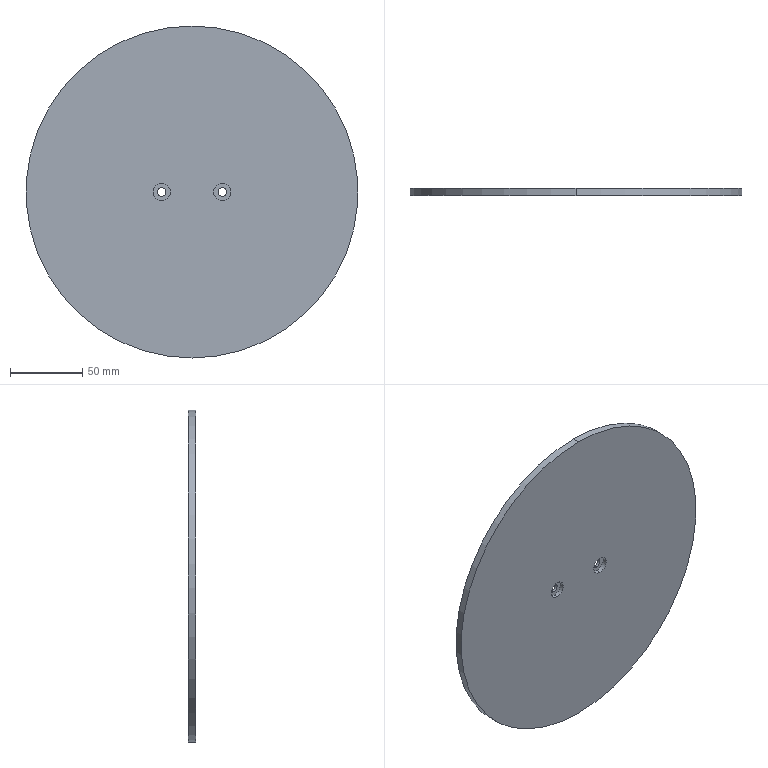Part | STEP file | Bottom cover | 1 solid | 14 faces | box 230 x 5 x 230 mm | volume 206946 mm3 | cylinder 10 | plane 4 | commonest cylinder face diameters 6 x4 12 x4 230 x2
STEP:
#1=CARTESIAN_POINT('',(21.,3.,6.));
#2=VERTEX_POINT('',#1);
#3=CARTESIAN_POINT('',(21.,3.,-6.));
#4=VERTEX_POINT('',#3);
#5=CARTESIAN_POINT('',(21.,3.,0.));
#6=DIRECTION('',(0.,-1.,0.));
#7=DIRECTION('',(0.,0.,-1.));
#8=AXIS2_PLACEMENT_3D('',#5,#6,#7);
#9=CIRCLE('',#8,6.);
#10=EDGE_CURVE('',#2,#4,#9,.T.);
#11=ORIENTED_EDGE('',*,*,#10,.F.);
#12=CARTESIAN_POINT('',(21.,0.,6.));
#13=VERTEX_POINT('',#12);
#14=CARTESIAN_POINT('',(21.,3.,6.));
#15=DIRECTION('',(0.,-1.,0.));
#16=VECTOR('',#15,1000.);
#17=LINE('',#14,#16);
#18=EDGE_CURVE('',#2,#13,#17,.T.);
#19=ORIENTED_EDGE('',*,*,#18,.T.);
#20=CARTESIAN_POINT('',(21.,0.,-6.));
#21=VERTEX_POINT('',#20);
#22=CARTESIAN_POINT('',(21.,0.,0.));
#23=DIRECTION('',(0.,-1.,0.));
#24=DIRECTION('',(0.,0.,-1.));
#25=AXIS2_PLACEMENT_3D('',#22,#23,#24);
#26=CIRCLE('',#25,6.);
#27=EDGE_CURVE('',#13,#21,#26,.T.);
#28=ORIENTED_EDGE('',*,*,#27,.T.);
#29=CARTESIAN_POINT('',(21.,3.,-6.));
#30=DIRECTION('',(0.,-1.,0.));
#31=VECTOR('',#30,1000.);
#32=LINE('',#29,#31);
#33=EDGE_CURVE('',#4,#21,#32,.T.);
#34=ORIENTED_EDGE('',*,*,#33,.F.);
#35=EDGE_LOOP('',(#11,#19,#28,#34));
#36=FACE_OUTER_BOUND('',#35,.T.);
#37=CARTESIAN_POINT('',(21.,3.,0.));
#38=DIRECTION('',(0.,-1.,0.));
#39=DIRECTION('',(0.,0.,-1.));
#40=AXIS2_PLACEMENT_3D('',#37,#38,#39);
#41=CYLINDRICAL_SURFACE('',#40,6.);
#42=ADVANCED_FACE('',(#36),#41,.F.);
#43=CARTESIAN_POINT('',(-21.,3.,6.));
#44=VERTEX_POINT('',#43);
#45=CARTESIAN_POINT('',(-21.,3.,-6.));
#46=VERTEX_POINT('',#45);
#47=CARTESIAN_POINT('',(-21.,3.,0.));
#48=DIRECTION('',(0.,-1.,0.));
#49=DIRECTION('',(0.,0.,-1.));
#50=AXIS2_PLACEMENT_3D('',#47,#48,#49);
#51=CIRCLE('',#50,6.);
#52=EDGE_CURVE('',#44,#46,#51,.T.);
#53=ORIENTED_EDGE('',*,*,#52,.F.);
#54=CARTESIAN_POINT('',(-21.,0.,6.));
#55=VERTEX_POINT('',#54);
#56=CARTESIAN_POINT('',(-21.,3.,6.));
#57=DIRECTION('',(0.,-1.,0.));
#58=VECTOR('',#57,1000.);
#59=LINE('',#56,#58);
#60=EDGE_CURVE('',#44,#55,#59,.T.);
#61=ORIENTED_EDGE('',*,*,#60,.T.);
#62=CARTESIAN_POINT('',(-21.,0.,-6.));
#63=VERTEX_POINT('',#62);
#64=CARTESIAN_POINT('',(-21.,0.,0.));
#65=DIRECTION('',(0.,-1.,0.));
#66=DIRECTION('',(0.,0.,-1.));
#67=AXIS2_PLACEMENT_3D('',#64,#65,#66);
#68=CIRCLE('',#67,6.);
#69=EDGE_CURVE('',#55,#63,#68,.T.);
#70=ORIENTED_EDGE('',*,*,#69,.T.);
#71=CARTESIAN_POINT('',(-21.,3.,-6.));
#72=DIRECTION('',(0.,-1.,0.));
#73=VECTOR('',#72,1000.);
#74=LINE('',#71,#73);
#75=EDGE_CURVE('',#46,#63,#74,.T.);
#76=ORIENTED_EDGE('',*,*,#75,.F.);
#77=EDGE_LOOP('',(#53,#61,#70,#76));
#78=FACE_OUTER_BOUND('',#77,.T.);
#79=CARTESIAN_POINT('',(-21.,3.,0.));
#80=DIRECTION('',(0.,-1.,0.));
#81=DIRECTION('',(0.,0.,-1.));
#82=AXIS2_PLACEMENT_3D('',#79,#80,#81);
#83=CYLINDRICAL_SURFACE('',#82,6.);
#84=ADVANCED_FACE('',(#78),#83,.F.);
#85=CARTESIAN_POINT('',(0.,5.,115.));
#86=VERTEX_POINT('',#85);
#87=CARTESIAN_POINT('',(0.,5.,-115.));
#88=VERTEX_POINT('',#87);
#89=CARTESIAN_POINT('',(0.,5.,0.));
#90=DIRECTION('',(0.,1.,0.));
#91=DIRECTION('',(0.,0.,1.));
#92=AXIS2_PLACEMENT_3D('',#89,#90,#91);
#93=CIRCLE('',#92,115.);
#94=EDGE_CURVE('',#86,#88,#93,.T.);
#95=ORIENTED_EDGE('',*,*,#94,.F.);
#96=CARTESIAN_POINT('',(0.,0.,115.));
#97=VERTEX_POINT('',#96);
#98=CARTESIAN_POINT('',(0.,5.,115.));
#99=DIRECTION('',(0.,-1.,0.));
#100=VECTOR('',#99,1000.);
#101=LINE('',#98,#100);
#102=EDGE_CURVE('',#86,#97,#101,.T.);
#103=ORIENTED_EDGE('',*,*,#102,.T.);
#104=CARTESIAN_POINT('',(0.,0.,-115.));
#105=VERTEX_POINT('',#104);
#106=CARTESIAN_POINT('',(0.,0.,0.));
#107=DIRECTION('',(0.,1.,0.));
#108=DIRECTION('',(0.,0.,1.));
#109=AXIS2_PLACEMENT_3D('',#106,#107,#108);
#110=CIRCLE('',#109,115.);
#111=EDGE_CURVE('',#97,#105,#110,.T.);
#112=ORIENTED_EDGE('',*,*,#111,.T.);
#113=CARTESIAN_POINT('',(0.,5.,-115.));
#114=DIRECTION('',(0.,-1.,0.));
#115=VECTOR('',#114,1000.);
#116=LINE('',#113,#115);
#117=EDGE_CURVE('',#88,#105,#116,.T.);
#118=ORIENTED_EDGE('',*,*,#117,.F.);
#119=EDGE_LOOP('',(#95,#103,#112,#118));
#120=FACE_OUTER_BOUND('',#119,.T.);
#121=CARTESIAN_POINT('',(0.,5.,0.));
#122=DIRECTION('',(0.,-1.,0.));
#123=DIRECTION('',(0.,0.,-1.));
#124=AXIS2_PLACEMENT_3D('',#121,#122,#123);
#125=CYLINDRICAL_SURFACE('',#124,115.);
#126=ADVANCED_FACE('',(#120),#125,.T.);
#127=CARTESIAN_POINT('',(-21.,3.,-3.));
#128=VERTEX_POINT('',#127);
#129=CARTESIAN_POINT('',(-21.,3.,3.));
#130=VERTEX_POINT('',#129);
#131=CARTESIAN_POINT('',(-21.,3.,0.));
#132=DIRECTION('',(0.,1.,0.));
#133=DIRECTION('',(0.,0.,-1.));
#134=AXIS2_PLACEMENT_3D('',#131,#132,#133);
#135=CIRCLE('',#134,3.);
#136=EDGE_CURVE('',#128,#130,#135,.T.);
#137=ORIENTED_EDGE('',*,*,#136,.F.);
#138=CARTESIAN_POINT('',(-21.,5.,-3.));
#139=VERTEX_POINT('',#138);
#140=CARTESIAN_POINT('',(-21.,-15.,-3.));
#141=DIRECTION('',(0.,1.,0.));
#142=VECTOR('',#141,1000.);
#143=LINE('',#140,#142);
#144=EDGE_CURVE('',#128,#139,#143,.T.);
#145=ORIENTED_EDGE('',*,*,#144,.T.);
#146=CARTESIAN_POINT('',(-21.,5.,3.));
#147=VERTEX_POINT('',#146);
#148=CARTESIAN_POINT('',(-21.,5.,0.));
#149=DIRECTION('',(0.,1.,0.));
#150=DIRECTION('',(0.,0.,1.));
#151=AXIS2_PLACEMENT_3D('',#148,#149,#150);
#152=CIRCLE('',#151,3.);
#153=EDGE_CURVE('',#139,#147,#152,.T.);
#154=ORIENTED_EDGE('',*,*,#153,.T.);
#155=CARTESIAN_POINT('',(-21.,-15.,3.));
#156=DIRECTION('',(0.,1.,0.));
#157=VECTOR('',#156,1000.);
#158=LINE('',#155,#157);
#159=EDGE_CURVE('',#130,#147,#158,.T.);
#160=ORIENTED_EDGE('',*,*,#159,.F.);
#161=EDGE_LOOP('',(#137,#145,#154,#160));
#162=FACE_OUTER_BOUND('',#161,.T.);
#163=CARTESIAN_POINT('',(-21.,-15.,0.));
#164=DIRECTION('',(0.,1.,0.));
#165=DIRECTION('',(0.,0.,1.));
#166=AXIS2_PLACEMENT_3D('',#163,#164,#165);
#167=CYLINDRICAL_SURFACE('',#166,3.);
#168=ADVANCED_FACE('',(#162),#167,.F.);
#169=CARTESIAN_POINT('',(21.,3.,-3.));
#170=VERTEX_POINT('',#169);
#171=CARTESIAN_POINT('',(21.,3.,3.));
#172=VERTEX_POINT('',#171);
#173=CARTESIAN_POINT('',(21.,3.,0.));
#174=DIRECTION('',(0.,1.,0.));
#175=DIRECTION('',(0.,0.,-1.));
#176=AXIS2_PLACEMENT_3D('',#173,#174,#175);
#177=CIRCLE('',#176,3.);
#178=EDGE_CURVE('',#170,#172,#177,.T.);
#179=ORIENTED_EDGE('',*,*,#178,.F.);
#180=CARTESIAN_POINT('',(21.,5.,-3.));
#181=VERTEX_POINT('',#180);
#182=CARTESIAN_POINT('',(21.,-15.,-3.));
#183=DIRECTION('',(0.,1.,0.));
#184=VECTOR('',#183,1000.);
#185=LINE('',#182,#184);
#186=EDGE_CURVE('',#170,#181,#185,.T.);
#187=ORIENTED_EDGE('',*,*,#186,.T.);
#188=CARTESIAN_POINT('',(21.,5.,3.));
#189=VERTEX_POINT('',#188);
#190=CARTESIAN_POINT('',(21.,5.,0.));
#191=DIRECTION('',(0.,1.,0.));
#192=DIRECTION('',(0.,0.,1.));
#193=AXIS2_PLACEMENT_3D('',#190,#191,#192);
#194=CIRCLE('',#193,3.);
#195=EDGE_CURVE('',#181,#189,#194,.T.);
#196=ORIENTED_EDGE('',*,*,#195,.T.);
#197=CARTESIAN_POINT('',(21.,-15.,3.));
#198=DIRECTION('',(0.,1.,0.));
#199=VECTOR('',#198,1000.);
#200=LINE('',#197,#199);
#201=EDGE_CURVE('',#172,#189,#200,.T.);
#202=ORIENTED_EDGE('',*,*,#201,.F.);
#203=EDGE_LOOP('',(#179,#187,#196,#202));
#204=FACE_OUTER_BOUND('',#203,.T.);
#205=CARTESIAN_POINT('',(21.,-15.,0.));
#206=DIRECTION('',(0.,1.,0.));
#207=DIRECTION('',(0.,0.,1.));
#208=AXIS2_PLACEMENT_3D('',#205,#206,#207);
#209=CYLINDRICAL_SURFACE('',#208,3.);
#210=ADVANCED_FACE('',(#204),#209,.F.);
#211=ORIENTED_EDGE('',*,*,#186,.F.);
#212=CARTESIAN_POINT('',(21.,3.,0.));
#213=DIRECTION('',(0.,1.,0.));
#214=DIRECTION('',(0.,0.,-1.));
#215=AXIS2_PLACEMENT_3D('',#212,#213,#214);
#216=CIRCLE('',#215,3.);
#217=EDGE_CURVE('',#172,#170,#216,.T.);
#218=ORIENTED_EDGE('',*,*,#217,.F.);
#219=ORIENTED_EDGE('',*,*,#201,.T.);
#220=CARTESIAN_POINT('',(21.,5.,0.));
#221=DIRECTION('',(0.,1.,0.));
#222=DIRECTION('',(0.,0.,1.));
#223=AXIS2_PLACEMENT_3D('',#220,#221,#222);
#224=CIRCLE('',#223,3.);
#225=EDGE_CURVE('',#189,#181,#224,.T.);
#226=ORIENTED_EDGE('',*,*,#225,.T.);
#227=EDGE_LOOP('',(#211,#218,#219,#226));
#228=FACE_OUTER_BOUND('',#227,.T.);
#229=CARTESIAN_POINT('',(21.,-15.,0.));
#230=DIRECTION('',(0.,1.,0.));
#231=DIRECTION('',(0.,0.,1.));
#232=AXIS2_PLACEMENT_3D('',#229,#230,#231);
#233=CYLINDRICAL_SURFACE('',#232,3.);
#234=ADVANCED_FACE('',(#228),#233,.F.);
#235=ORIENTED_EDGE('',*,*,#144,.F.);
#236=CARTESIAN_POINT('',(-21.,3.,0.));
#237=DIRECTION('',(0.,1.,0.));
#238=DIRECTION('',(0.,0.,-1.));
#239=AXIS2_PLACEMENT_3D('',#236,#237,#238);
#240=CIRCLE('',#239,3.);
#241=EDGE_CURVE('',#130,#128,#240,.T.);
#242=ORIENTED_EDGE('',*,*,#241,.F.);
#243=ORIENTED_EDGE('',*,*,#159,.T.);
#244=CARTESIAN_POINT('',(-21.,5.,0.));
#245=DIRECTION('',(0.,1.,0.));
#246=DIRECTION('',(0.,0.,1.));
#247=AXIS2_PLACEMENT_3D('',#244,#245,#246);
#248=CIRCLE('',#247,3.);
#249=EDGE_CURVE('',#147,#139,#248,.T.);
#250=ORIENTED_EDGE('',*,*,#249,.T.);
#251=EDGE_LOOP('',(#235,#242,#243,#250));
#252=FACE_OUTER_BOUND('',#251,.T.);
#253=CARTESIAN_POINT('',(-21.,-15.,0.));
#254=DIRECTION('',(0.,1.,0.));
#255=DIRECTION('',(0.,0.,1.));
#256=AXIS2_PLACEMENT_3D('',#253,#254,#255);
#257=CYLINDRICAL_SURFACE('',#256,3.);
#258=ADVANCED_FACE('',(#252),#257,.F.);
#259=ORIENTED_EDGE('',*,*,#102,.F.);
#260=CARTESIAN_POINT('',(0.,5.,0.));
#261=DIRECTION('',(0.,1.,0.));
#262=DIRECTION('',(0.,0.,1.));
#263=AXIS2_PLACEMENT_3D('',#260,#261,#262);
#264=CIRCLE('',#263,115.);
#265=EDGE_CURVE('',#88,#86,#264,.T.);
#266=ORIENTED_EDGE('',*,*,#265,.F.);
#267=ORIENTED_EDGE('',*,*,#117,.T.);
#268=CARTESIAN_POINT('',(0.,0.,0.));
#269=DIRECTION('',(0.,1.,0.));
#270=DIRECTION('',(0.,0.,1.));
#271=AXIS2_PLACEMENT_3D('',#268,#269,#270);
#272=CIRCLE('',#271,115.);
#273=EDGE_CURVE('',#105,#97,#272,.T.);
#274=ORIENTED_EDGE('',*,*,#273,.T.);
#275=EDGE_LOOP('',(#259,#266,#267,#274));
#276=FACE_OUTER_BOUND('',#275,.T.);
#277=CARTESIAN_POINT('',(0.,5.,0.));
#278=DIRECTION('',(0.,-1.,0.));
#279=DIRECTION('',(0.,0.,-1.));
#280=AXIS2_PLACEMENT_3D('',#277,#278,#279);
#281=CYLINDRICAL_SURFACE('',#280,115.);
#282=ADVANCED_FACE('',(#276),#281,.T.);
#283=ORIENTED_EDGE('',*,*,#249,.F.);
#284=ORIENTED_EDGE('',*,*,#153,.F.);
#285=EDGE_LOOP('',(#283,#284));
#286=FACE_BOUND('',#285,.T.);
#287=ORIENTED_EDGE('',*,*,#225,.F.);
#288=ORIENTED_EDGE('',*,*,#195,.F.);
#289=EDGE_LOOP('',(#287,#288));
#290=FACE_BOUND('',#289,.T.);
#291=ORIENTED_EDGE('',*,*,#265,.T.);
#292=ORIENTED_EDGE('',*,*,#94,.T.);
#293=EDGE_LOOP('',(#291,#292));
#294=FACE_OUTER_BOUND('',#293,.T.);
#295=CARTESIAN_POINT('',(0.,5.,0.));
#296=DIRECTION('',(0.,1.,0.));
#297=DIRECTION('',(0.,0.,1.));
#298=AXIS2_PLACEMENT_3D('',#295,#296,#297);
#299=PLANE('',#298);
#300=ADVANCED_FACE('',(#286,#290,#294),#299,.T.);
#301=CARTESIAN_POINT('',(-21.,0.,0.));
#302=DIRECTION('',(0.,-1.,0.));
#303=DIRECTION('',(0.,0.,-1.));
#304=AXIS2_PLACEMENT_3D('',#301,#302,#303);
#305=CIRCLE('',#304,6.);
#306=EDGE_CURVE('',#63,#55,#305,.T.);
#307=ORIENTED_EDGE('',*,*,#306,.F.);
#308=ORIENTED_EDGE('',*,*,#69,.F.);
#309=EDGE_LOOP('',(#307,#308));
#310=FACE_BOUND('',#309,.T.);
#311=CARTESIAN_POINT('',(21.,0.,0.));
#312=DIRECTION('',(0.,-1.,0.));
#313=DIRECTION('',(0.,0.,-1.));
#314=AXIS2_PLACEMENT_3D('',#311,#312,#313);
#315=CIRCLE('',#314,6.);
#316=EDGE_CURVE('',#21,#13,#315,.T.);
#317=ORIENTED_EDGE('',*,*,#316,.F.);
#318=ORIENTED_EDGE('',*,*,#27,.F.);
#319=EDGE_LOOP('',(#317,#318));
#320=FACE_BOUND('',#319,.T.);
#321=ORIENTED_EDGE('',*,*,#273,.F.);
#322=ORIENTED_EDGE('',*,*,#111,.F.);
#323=EDGE_LOOP('',(#321,#322));
#324=FACE_OUTER_BOUND('',#323,.T.);
#325=CARTESIAN_POINT('',(0.,0.,0.));
#326=DIRECTION('',(0.,1.,0.));
#327=DIRECTION('',(0.,0.,1.));
#328=AXIS2_PLACEMENT_3D('',#325,#326,#327);
#329=PLANE('',#328);
#330=ADVANCED_FACE('',(#310,#320,#324),#329,.F.);
#331=CARTESIAN_POINT('',(-21.,3.,0.));
#332=DIRECTION('',(0.,-1.,0.));
#333=DIRECTION('',(0.,0.,-1.));
#334=AXIS2_PLACEMENT_3D('',#331,#332,#333);
#335=CIRCLE('',#334,6.);
#336=EDGE_CURVE('',#46,#44,#335,.T.);
#337=ORIENTED_EDGE('',*,*,#336,.T.);
#338=ORIENTED_EDGE('',*,*,#52,.T.);
#339=EDGE_LOOP('',(#337,#338));
#340=FACE_OUTER_BOUND('',#339,.T.);
#341=ORIENTED_EDGE('',*,*,#241,.T.);
#342=ORIENTED_EDGE('',*,*,#136,.T.);
#343=EDGE_LOOP('',(#341,#342));
#344=FACE_BOUND('',#343,.T.);
#345=CARTESIAN_POINT('',(-21.,3.,0.));
#346=DIRECTION('',(0.,-1.,0.));
#347=DIRECTION('',(0.,0.,-1.));
#348=AXIS2_PLACEMENT_3D('',#345,#346,#347);
#349=PLANE('',#348);
#350=ADVANCED_FACE('',(#340,#344),#349,.T.);
#351=ORIENTED_EDGE('',*,*,#60,.F.);
#352=ORIENTED_EDGE('',*,*,#336,.F.);
#353=ORIENTED_EDGE('',*,*,#75,.T.);
#354=ORIENTED_EDGE('',*,*,#306,.T.);
#355=EDGE_LOOP('',(#351,#352,#353,#354));
#356=FACE_OUTER_BOUND('',#355,.T.);
#357=CARTESIAN_POINT('',(-21.,3.,0.));
#358=DIRECTION('',(0.,-1.,0.));
#359=DIRECTION('',(0.,0.,-1.));
#360=AXIS2_PLACEMENT_3D('',#357,#358,#359);
#361=CYLINDRICAL_SURFACE('',#360,6.);
#362=ADVANCED_FACE('',(#356),#361,.F.);
#363=CARTESIAN_POINT('',(21.,3.,0.));
#364=DIRECTION('',(0.,-1.,0.));
#365=DIRECTION('',(0.,0.,-1.));
#366=AXIS2_PLACEMENT_3D('',#363,#364,#365);
#367=CIRCLE('',#366,6.);
#368=EDGE_CURVE('',#4,#2,#367,.T.);
#369=ORIENTED_EDGE('',*,*,#368,.T.);
#370=ORIENTED_EDGE('',*,*,#10,.T.);
#371=EDGE_LOOP('',(#369,#370));
#372=FACE_OUTER_BOUND('',#371,.T.);
#373=ORIENTED_EDGE('',*,*,#217,.T.);
#374=ORIENTED_EDGE('',*,*,#178,.T.);
#375=EDGE_LOOP('',(#373,#374));
#376=FACE_BOUND('',#375,.T.);
#377=CARTESIAN_POINT('',(21.,3.,0.));
#378=DIRECTION('',(0.,-1.,0.));
#379=DIRECTION('',(0.,0.,-1.));
#380=AXIS2_PLACEMENT_3D('',#377,#378,#379);
#381=PLANE('',#380);
#382=ADVANCED_FACE('',(#372,#376),#381,.T.);
#383=ORIENTED_EDGE('',*,*,#18,.F.);
#384=ORIENTED_EDGE('',*,*,#368,.F.);
#385=ORIENTED_EDGE('',*,*,#33,.T.);
#386=ORIENTED_EDGE('',*,*,#316,.T.);
#387=EDGE_LOOP('',(#383,#384,#385,#386));
#388=FACE_OUTER_BOUND('',#387,.T.);
#389=CARTESIAN_POINT('',(21.,3.,0.));
#390=DIRECTION('',(0.,-1.,0.));
#391=DIRECTION('',(0.,0.,-1.));
#392=AXIS2_PLACEMENT_3D('',#389,#390,#391);
#393=CYLINDRICAL_SURFACE('',#392,6.);
#394=ADVANCED_FACE('',(#388),#393,.F.);
#395=CLOSED_SHELL('',(#42,#84,#126,#168,#210,#234,#258,#282,#300,#330,#350,#362,#382,#394));
#396=MANIFOLD_SOLID_BREP('',#395);
#397=CARTESIAN_POINT('',(0.,0.,0.));
#398=DIRECTION('',(0.,0.,1.));
#399=DIRECTION('',(1.,0.,0.));
#400=AXIS2_PLACEMENT_3D('',#397,#398,#399);
#401=(LENGTH_UNIT()NAMED_UNIT(*)SI_UNIT(.MILLI.,.METRE.));
#402=UNCERTAINTY_MEASURE_WITH_UNIT(LENGTH_MEASURE(0.00001),#401,'','');
#403=(NAMED_UNIT(*)PLANE_ANGLE_UNIT()SI_UNIT($,.RADIAN.));
#404=(NAMED_UNIT(*)SI_UNIT($,.STERADIAN.)SOLID_ANGLE_UNIT());
#405=(GEOMETRIC_REPRESENTATION_CONTEXT(3)GLOBAL_UNCERTAINTY_ASSIGNED_CONTEXT((#402))GLOBAL_UNIT_ASSIGNED_CONTEXT((#401,#403,#404))REPRESENTATION_CONTEXT('',''));
#406=ADVANCED_BREP_SHAPE_REPRESENTATION('',(#396,#400),#405);